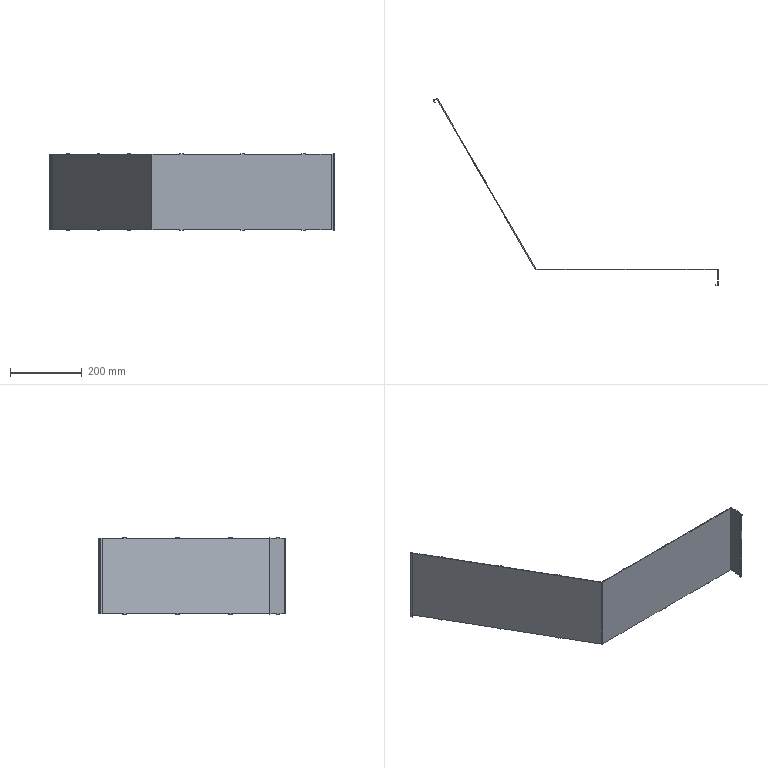Part | STEP file | zh005 | 1 solid | 86 faces | box 791.755 x 520.982 x 214 mm | volume 471579 mm3 | plane 74 | cylinder 12 | commonest cylinder face diameters 1 x6 5 x6